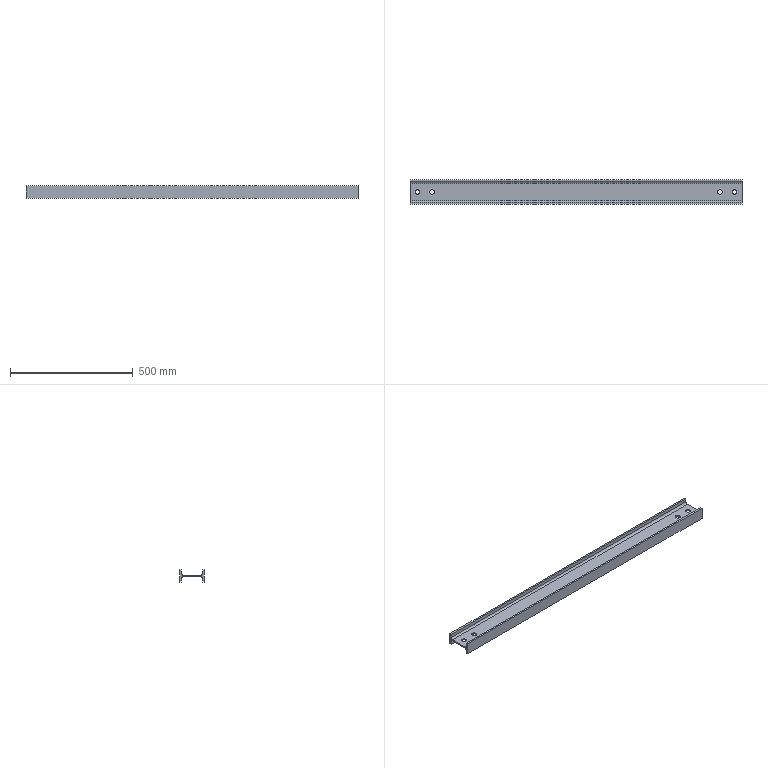Part | STEP file | 休息台辅梁1主体_Default<As Machined> | 1 solid | 26 faces | box 1350 x 100 x 50 mm | volume 1593996 mm3 | plane 14 | cylinder 12 | commonest cylinder face diameters 19 x8 16 x4